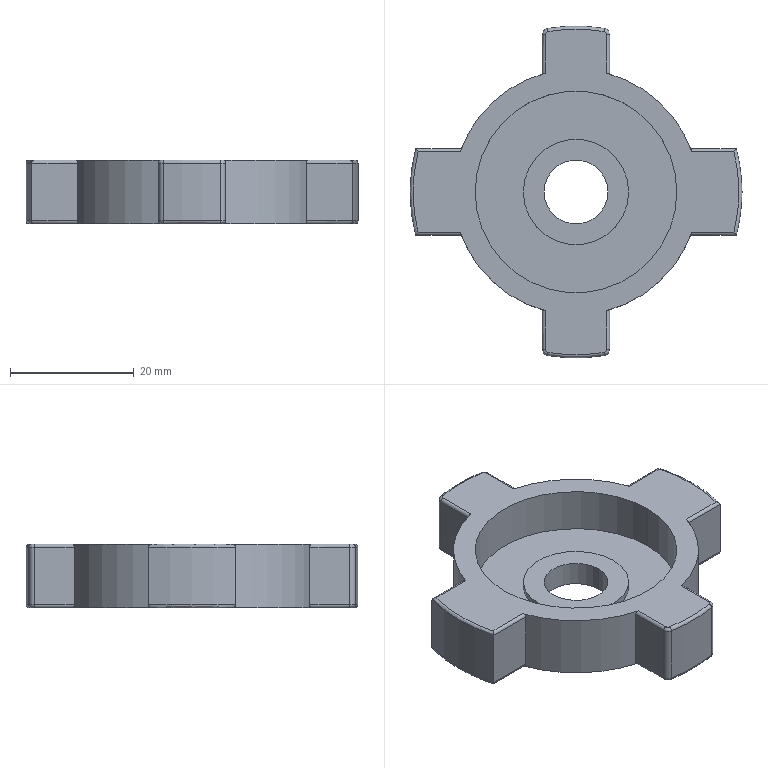Part | SolidWorks | features BaseBody 1 | 1 solid | 63 faces | box 53.657 x 53.657 x 10.33 mm | volume 10160 mm3 | cylinder 35 | spline 16 | plane 12 | commonest cylinder face diameters 1.003 x12 53.657 x5 0.98 x4 1.961 x4 39.616 x4 10.33 x2